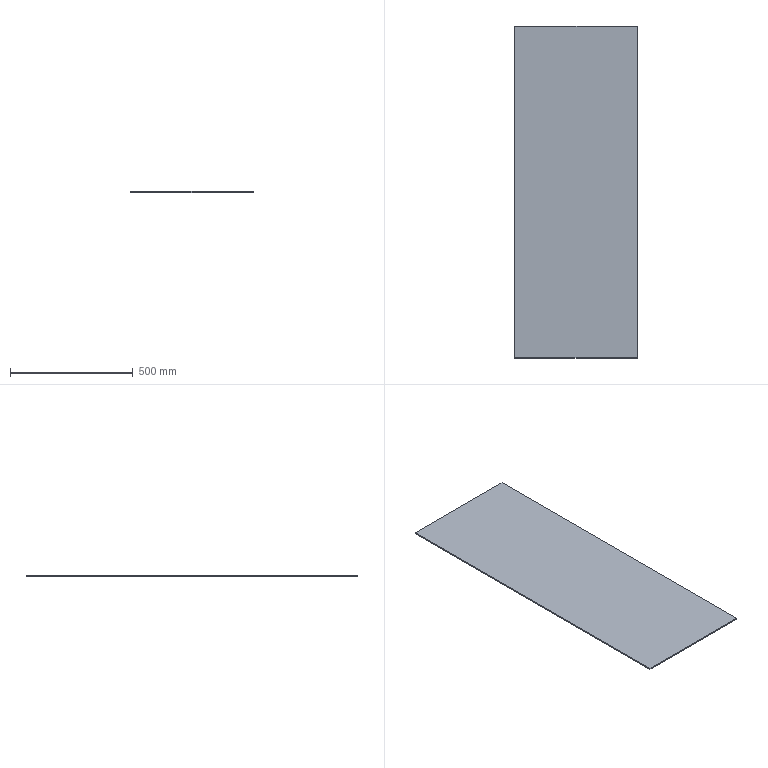Part | SolidWorks | features Extrusion 1, HoleWzd 1 | 1 solid | 6 faces | box 499 x 1350 x 5 mm | volume 3368250 mm3 | plane 6
STEP:
#1=CARTESIAN_POINT('',(249.5,-675.,0.));
#2=VERTEX_POINT('',#1);
#3=CARTESIAN_POINT('',(249.5,675.,0.));
#4=VERTEX_POINT('',#3);
#5=CARTESIAN_POINT('',(249.5,675.,0.));
#6=DIRECTION('',(0.,1.,0.));
#7=VECTOR('',#6,1000.);
#8=LINE('',#5,#7);
#9=EDGE_CURVE('',#2,#4,#8,.T.);
#10=ORIENTED_EDGE('',*,*,#9,.T.);
#11=CARTESIAN_POINT('',(249.5,675.,5.));
#12=VERTEX_POINT('',#11);
#13=CARTESIAN_POINT('',(249.5,675.,5.));
#14=DIRECTION('',(0.,0.,-1.));
#15=VECTOR('',#14,1000.);
#16=LINE('',#13,#15);
#17=EDGE_CURVE('',#12,#4,#16,.T.);
#18=ORIENTED_EDGE('',*,*,#17,.F.);
#19=CARTESIAN_POINT('',(249.5,-675.,5.));
#20=VERTEX_POINT('',#19);
#21=CARTESIAN_POINT('',(249.5,675.,5.));
#22=DIRECTION('',(0.,1.,0.));
#23=VECTOR('',#22,1000.);
#24=LINE('',#21,#23);
#25=EDGE_CURVE('',#20,#12,#24,.T.);
#26=ORIENTED_EDGE('',*,*,#25,.F.);
#27=CARTESIAN_POINT('',(249.5,-675.,5.));
#28=DIRECTION('',(0.,0.,-1.));
#29=VECTOR('',#28,1000.);
#30=LINE('',#27,#29);
#31=EDGE_CURVE('',#20,#2,#30,.T.);
#32=ORIENTED_EDGE('',*,*,#31,.T.);
#33=EDGE_LOOP('',(#10,#18,#26,#32));
#34=FACE_OUTER_BOUND('',#33,.T.);
#35=CARTESIAN_POINT('',(249.5,675.,5.));
#36=DIRECTION('',(-1.,0.,0.));
#37=DIRECTION('',(0.,-1.,0.));
#38=AXIS2_PLACEMENT_3D('',#35,#36,#37);
#39=PLANE('',#38);
#40=ADVANCED_FACE('',(#34),#39,.F.);
#41=CARTESIAN_POINT('',(-249.5,675.,0.));
#42=VERTEX_POINT('',#41);
#43=CARTESIAN_POINT('',(-249.5,675.,0.));
#44=DIRECTION('',(-1.,0.,0.));
#45=VECTOR('',#44,1000.);
#46=LINE('',#43,#45);
#47=EDGE_CURVE('',#4,#42,#46,.T.);
#48=ORIENTED_EDGE('',*,*,#47,.T.);
#49=CARTESIAN_POINT('',(-249.5,675.,5.));
#50=VERTEX_POINT('',#49);
#51=CARTESIAN_POINT('',(-249.5,675.,5.));
#52=DIRECTION('',(0.,0.,-1.));
#53=VECTOR('',#52,1000.);
#54=LINE('',#51,#53);
#55=EDGE_CURVE('',#50,#42,#54,.T.);
#56=ORIENTED_EDGE('',*,*,#55,.F.);
#57=CARTESIAN_POINT('',(-249.5,675.,5.));
#58=DIRECTION('',(-1.,0.,0.));
#59=VECTOR('',#58,1000.);
#60=LINE('',#57,#59);
#61=EDGE_CURVE('',#12,#50,#60,.T.);
#62=ORIENTED_EDGE('',*,*,#61,.F.);
#63=ORIENTED_EDGE('',*,*,#17,.T.);
#64=EDGE_LOOP('',(#48,#56,#62,#63));
#65=FACE_OUTER_BOUND('',#64,.T.);
#66=CARTESIAN_POINT('',(-249.5,675.,5.));
#67=DIRECTION('',(0.,-1.,0.));
#68=DIRECTION('',(0.,0.,-1.));
#69=AXIS2_PLACEMENT_3D('',#66,#67,#68);
#70=PLANE('',#69);
#71=ADVANCED_FACE('',(#65),#70,.F.);
#72=CARTESIAN_POINT('',(-249.5,-675.,0.));
#73=VERTEX_POINT('',#72);
#74=CARTESIAN_POINT('',(-249.5,675.,0.));
#75=DIRECTION('',(0.,-1.,0.));
#76=VECTOR('',#75,1000.);
#77=LINE('',#74,#76);
#78=EDGE_CURVE('',#42,#73,#77,.T.);
#79=ORIENTED_EDGE('',*,*,#78,.T.);
#80=CARTESIAN_POINT('',(-249.5,-675.,5.));
#81=VERTEX_POINT('',#80);
#82=CARTESIAN_POINT('',(-249.5,-675.,5.));
#83=DIRECTION('',(0.,0.,-1.));
#84=VECTOR('',#83,1000.);
#85=LINE('',#82,#84);
#86=EDGE_CURVE('',#81,#73,#85,.T.);
#87=ORIENTED_EDGE('',*,*,#86,.F.);
#88=CARTESIAN_POINT('',(-249.5,675.,5.));
#89=DIRECTION('',(0.,-1.,0.));
#90=VECTOR('',#89,1000.);
#91=LINE('',#88,#90);
#92=EDGE_CURVE('',#50,#81,#91,.T.);
#93=ORIENTED_EDGE('',*,*,#92,.F.);
#94=ORIENTED_EDGE('',*,*,#55,.T.);
#95=EDGE_LOOP('',(#79,#87,#93,#94));
#96=FACE_OUTER_BOUND('',#95,.T.);
#97=CARTESIAN_POINT('',(-249.5,675.,5.));
#98=DIRECTION('',(1.,0.,0.));
#99=DIRECTION('',(0.,1.,0.));
#100=AXIS2_PLACEMENT_3D('',#97,#98,#99);
#101=PLANE('',#100);
#102=ADVANCED_FACE('',(#96),#101,.F.);
#103=CARTESIAN_POINT('',(-249.5,-675.,0.));
#104=DIRECTION('',(1.,0.,0.));
#105=VECTOR('',#104,1000.);
#106=LINE('',#103,#105);
#107=EDGE_CURVE('',#73,#2,#106,.T.);
#108=ORIENTED_EDGE('',*,*,#107,.T.);
#109=ORIENTED_EDGE('',*,*,#31,.F.);
#110=CARTESIAN_POINT('',(-249.5,-675.,5.));
#111=DIRECTION('',(1.,0.,0.));
#112=VECTOR('',#111,1000.);
#113=LINE('',#110,#112);
#114=EDGE_CURVE('',#81,#20,#113,.T.);
#115=ORIENTED_EDGE('',*,*,#114,.F.);
#116=ORIENTED_EDGE('',*,*,#86,.T.);
#117=EDGE_LOOP('',(#108,#109,#115,#116));
#118=FACE_OUTER_BOUND('',#117,.T.);
#119=CARTESIAN_POINT('',(-249.5,-675.,5.));
#120=DIRECTION('',(0.,1.,0.));
#121=DIRECTION('',(0.,0.,1.));
#122=AXIS2_PLACEMENT_3D('',#119,#120,#121);
#123=PLANE('',#122);
#124=ADVANCED_FACE('',(#118),#123,.F.);
#125=ORIENTED_EDGE('',*,*,#25,.T.);
#126=ORIENTED_EDGE('',*,*,#61,.T.);
#127=ORIENTED_EDGE('',*,*,#92,.T.);
#128=ORIENTED_EDGE('',*,*,#114,.T.);
#129=EDGE_LOOP('',(#125,#126,#127,#128));
#130=FACE_OUTER_BOUND('',#129,.T.);
#131=CARTESIAN_POINT('',(0.,0.,5.));
#132=DIRECTION('',(0.,0.,1.));
#133=DIRECTION('',(1.,0.,0.));
#134=AXIS2_PLACEMENT_3D('',#131,#132,#133);
#135=PLANE('',#134);
#136=ADVANCED_FACE('',(#130),#135,.T.);
#137=ORIENTED_EDGE('',*,*,#9,.F.);
#138=ORIENTED_EDGE('',*,*,#107,.F.);
#139=ORIENTED_EDGE('',*,*,#78,.F.);
#140=ORIENTED_EDGE('',*,*,#47,.F.);
#141=EDGE_LOOP('',(#137,#138,#139,#140));
#142=FACE_OUTER_BOUND('',#141,.T.);
#143=CARTESIAN_POINT('',(0.,0.,0.));
#144=DIRECTION('',(0.,0.,1.));
#145=DIRECTION('',(1.,0.,0.));
#146=AXIS2_PLACEMENT_3D('',#143,#144,#145);
#147=PLANE('',#146);
#148=ADVANCED_FACE('',(#142),#147,.F.);
#149=CLOSED_SHELL('',(#40,#71,#102,#124,#136,#148));
#150=MANIFOLD_SOLID_BREP('',#149);
#151=CARTESIAN_POINT('',(0.,0.,0.));
#152=DIRECTION('',(0.,0.,1.));
#153=DIRECTION('',(1.,0.,0.));
#154=AXIS2_PLACEMENT_3D('',#151,#152,#153);
#155=(LENGTH_UNIT()NAMED_UNIT(*)SI_UNIT(.MILLI.,.METRE.));
#156=UNCERTAINTY_MEASURE_WITH_UNIT(LENGTH_MEASURE(0.00001),#155,'','');
#157=(NAMED_UNIT(*)PLANE_ANGLE_UNIT()SI_UNIT($,.RADIAN.));
#158=(NAMED_UNIT(*)SI_UNIT($,.STERADIAN.)SOLID_ANGLE_UNIT());
#159=(GEOMETRIC_REPRESENTATION_CONTEXT(3)GLOBAL_UNCERTAINTY_ASSIGNED_CONTEXT((#156))GLOBAL_UNIT_ASSIGNED_CONTEXT((#155,#157,#158))REPRESENTATION_CONTEXT('',''));
#160=ADVANCED_BREP_SHAPE_REPRESENTATION('',(#150,#154),#159);